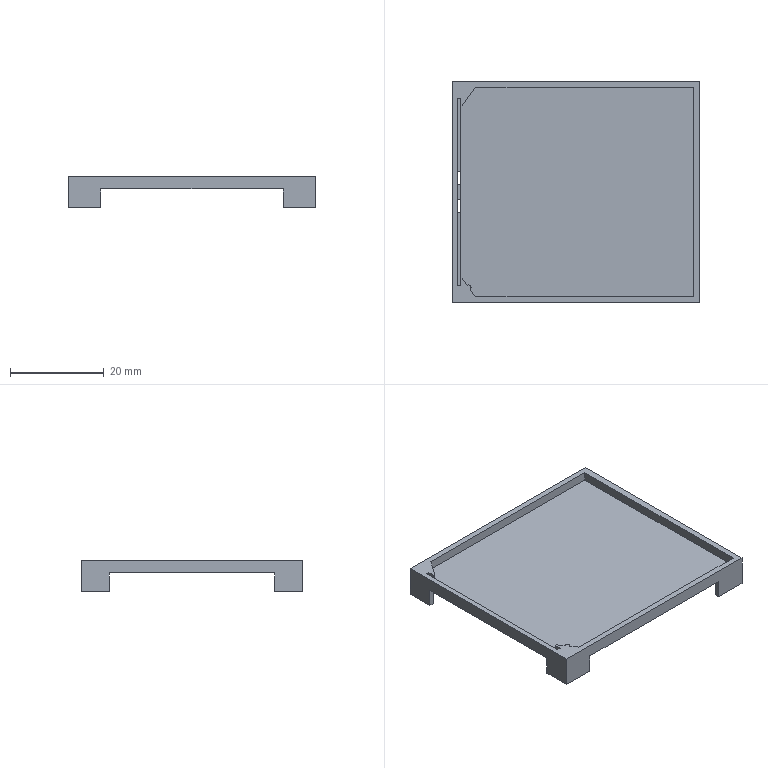Part | NX | features DATUM_CSYS 6, EXTRUDE 5, SKETCH 5 | 1 solid | 49 faces | box 53 x 47.4 x 6.67 mm | volume 2471 mm3 | plane 46 | cylinder 3 | commonest cylinder face diameters 0.4 x2 1 x1
STEP:
#1=CARTESIAN_POINT('',(1.15,25.4,0.35));
#2=VERTEX_POINT('',#1);
#3=CARTESIAN_POINT('',(1.85,25.4,0.35));
#4=VERTEX_POINT('',#3);
#5=CARTESIAN_POINT('',(1.15,25.4,0.35));
#6=DIRECTION('',(1.,0.,0.));
#7=VECTOR('',#6,1000.);
#8=LINE('',#5,#7);
#9=EDGE_CURVE('',#2,#4,#8,.T.);
#10=ORIENTED_EDGE('',*,*,#9,.F.);
#11=CARTESIAN_POINT('',(1.15,22.,0.35));
#12=VERTEX_POINT('',#11);
#13=CARTESIAN_POINT('',(1.15,43.6,0.35));
#14=DIRECTION('',(0.,-1.,0.));
#15=VECTOR('',#14,1000.);
#16=LINE('',#13,#15);
#17=EDGE_CURVE('',#2,#12,#16,.T.);
#18=ORIENTED_EDGE('',*,*,#17,.T.);
#19=CARTESIAN_POINT('',(1.85,22.,0.35));
#20=VERTEX_POINT('',#19);
#21=CARTESIAN_POINT('',(1.85,22.,0.35));
#22=DIRECTION('',(-1.,0.,0.));
#23=VECTOR('',#22,1000.);
#24=LINE('',#21,#23);
#25=EDGE_CURVE('',#20,#12,#24,.T.);
#26=ORIENTED_EDGE('',*,*,#25,.F.);
#27=CARTESIAN_POINT('',(1.85,3.8,0.35));
#28=DIRECTION('',(0.,1.,0.));
#29=VECTOR('',#28,1000.);
#30=LINE('',#27,#29);
#31=EDGE_CURVE('',#20,#4,#30,.T.);
#32=ORIENTED_EDGE('',*,*,#31,.T.);
#33=EDGE_LOOP('',(#10,#18,#26,#32));
#34=FACE_BOUND('',#33,.T.);
#35=CARTESIAN_POINT('',(0.,0.,0.35));
#36=DIRECTION('',(0.,0.,1.));
#37=DIRECTION('',(1.,0.,0.));
#38=AXIS2_PLACEMENT_3D('',#35,#36,#37);
#39=PLANE('',#38);
#40=ADVANCED_FACE('',(#34),#39,.T.);
#41=CARTESIAN_POINT('',(1.15,19.4,0.35));
#42=VERTEX_POINT('',#41);
#43=CARTESIAN_POINT('',(1.85,19.4,0.35));
#44=VERTEX_POINT('',#43);
#45=CARTESIAN_POINT('',(1.15,19.4,0.35));
#46=DIRECTION('',(1.,0.,0.));
#47=VECTOR('',#46,1000.);
#48=LINE('',#45,#47);
#49=EDGE_CURVE('',#42,#44,#48,.T.);
#50=ORIENTED_EDGE('',*,*,#49,.F.);
#51=CARTESIAN_POINT('',(1.15,3.8,0.35));
#52=VERTEX_POINT('',#51);
#53=CARTESIAN_POINT('',(1.15,43.6,0.35));
#54=DIRECTION('',(0.,-1.,0.));
#55=VECTOR('',#54,1000.);
#56=LINE('',#53,#55);
#57=EDGE_CURVE('',#42,#52,#56,.T.);
#58=ORIENTED_EDGE('',*,*,#57,.T.);
#59=CARTESIAN_POINT('',(1.85,3.8,0.35));
#60=VERTEX_POINT('',#59);
#61=CARTESIAN_POINT('',(1.15,3.8,0.35));
#62=DIRECTION('',(1.,0.,0.));
#63=VECTOR('',#62,1000.);
#64=LINE('',#61,#63);
#65=EDGE_CURVE('',#52,#60,#64,.T.);
#66=ORIENTED_EDGE('',*,*,#65,.T.);
#67=CARTESIAN_POINT('',(1.85,3.8,0.35));
#68=DIRECTION('',(0.,1.,0.));
#69=VECTOR('',#68,1000.);
#70=LINE('',#67,#69);
#71=EDGE_CURVE('',#60,#44,#70,.T.);
#72=ORIENTED_EDGE('',*,*,#71,.T.);
#73=EDGE_LOOP('',(#50,#58,#66,#72));
#74=FACE_BOUND('',#73,.T.);
#75=CARTESIAN_POINT('',(0.,0.,0.35));
#76=DIRECTION('',(0.,0.,1.));
#77=DIRECTION('',(1.,0.,0.));
#78=AXIS2_PLACEMENT_3D('',#75,#76,#77);
#79=PLANE('',#78);
#80=ADVANCED_FACE('',(#74),#79,.T.);
#81=CARTESIAN_POINT('',(1.85,28.,0.));
#82=VERTEX_POINT('',#81);
#83=CARTESIAN_POINT('',(1.15,28.,0.));
#84=VERTEX_POINT('',#83);
#85=CARTESIAN_POINT('',(0.,28.,0.));
#86=DIRECTION('',(-1.,0.,0.));
#87=VECTOR('',#86,1000.);
#88=LINE('',#85,#87);
#89=EDGE_CURVE('',#82,#84,#88,.T.);
#90=ORIENTED_EDGE('',*,*,#89,.T.);
#91=CARTESIAN_POINT('',(1.15,25.4,0.));
#92=VERTEX_POINT('',#91);
#93=CARTESIAN_POINT('',(1.15,0.,0.));
#94=DIRECTION('',(0.,-1.,0.));
#95=VECTOR('',#94,1000.);
#96=LINE('',#93,#95);
#97=EDGE_CURVE('',#84,#92,#96,.T.);
#98=ORIENTED_EDGE('',*,*,#97,.T.);
#99=CARTESIAN_POINT('',(1.85,25.4,0.));
#100=VERTEX_POINT('',#99);
#101=CARTESIAN_POINT('',(0.,25.4,0.));
#102=DIRECTION('',(1.,0.,0.));
#103=VECTOR('',#102,1000.);
#104=LINE('',#101,#103);
#105=EDGE_CURVE('',#92,#100,#104,.T.);
#106=ORIENTED_EDGE('',*,*,#105,.T.);
#107=CARTESIAN_POINT('',(1.85,0.,0.));
#108=DIRECTION('',(0.,1.,0.));
#109=VECTOR('',#108,1000.);
#110=LINE('',#107,#109);
#111=EDGE_CURVE('',#100,#82,#110,.T.);
#112=ORIENTED_EDGE('',*,*,#111,.T.);
#113=EDGE_LOOP('',(#90,#98,#106,#112));
#114=FACE_BOUND('',#113,.T.);
#115=CARTESIAN_POINT('',(1.85,22.,0.));
#116=VERTEX_POINT('',#115);
#117=CARTESIAN_POINT('',(1.15,22.,0.));
#118=VERTEX_POINT('',#117);
#119=CARTESIAN_POINT('',(0.,22.,0.));
#120=DIRECTION('',(-1.,0.,0.));
#121=VECTOR('',#120,1000.);
#122=LINE('',#119,#121);
#123=EDGE_CURVE('',#116,#118,#122,.T.);
#124=ORIENTED_EDGE('',*,*,#123,.T.);
#125=CARTESIAN_POINT('',(1.15,19.4,0.));
#126=VERTEX_POINT('',#125);
#127=CARTESIAN_POINT('',(1.15,0.,0.));
#128=DIRECTION('',(0.,-1.,0.));
#129=VECTOR('',#128,1000.);
#130=LINE('',#127,#129);
#131=EDGE_CURVE('',#118,#126,#130,.T.);
#132=ORIENTED_EDGE('',*,*,#131,.T.);
#133=CARTESIAN_POINT('',(1.85,19.4,0.));
#134=VERTEX_POINT('',#133);
#135=CARTESIAN_POINT('',(0.,19.4,0.));
#136=DIRECTION('',(1.,0.,0.));
#137=VECTOR('',#136,1000.);
#138=LINE('',#135,#137);
#139=EDGE_CURVE('',#126,#134,#138,.T.);
#140=ORIENTED_EDGE('',*,*,#139,.T.);
#141=CARTESIAN_POINT('',(1.85,0.,0.));
#142=DIRECTION('',(0.,1.,0.));
#143=VECTOR('',#142,1000.);
#144=LINE('',#141,#143);
#145=EDGE_CURVE('',#134,#116,#144,.T.);
#146=ORIENTED_EDGE('',*,*,#145,.T.);
#147=EDGE_LOOP('',(#124,#132,#140,#146));
#148=FACE_BOUND('',#147,.T.);
#149=CARTESIAN_POINT('',(46.,46.4,0.));
#150=VERTEX_POINT('',#149);
#151=CARTESIAN_POINT('',(46.,47.4,0.));
#152=VERTEX_POINT('',#151);
#153=CARTESIAN_POINT('',(46.,46.4,0.));
#154=DIRECTION('',(0.,1.,0.));
#155=VECTOR('',#154,1000.);
#156=LINE('',#153,#155);
#157=EDGE_CURVE('',#150,#152,#156,.T.);
#158=ORIENTED_EDGE('',*,*,#157,.F.);
#159=CARTESIAN_POINT('',(52.,46.4,0.));
#160=VERTEX_POINT('',#159);
#161=CARTESIAN_POINT('',(52.,46.4,0.));
#162=DIRECTION('',(-1.,0.,0.));
#163=VECTOR('',#162,1000.);
#164=LINE('',#161,#163);
#165=EDGE_CURVE('',#160,#150,#164,.T.);
#166=ORIENTED_EDGE('',*,*,#165,.F.);
#167=CARTESIAN_POINT('',(52.,41.4,0.));
#168=VERTEX_POINT('',#167);
#169=CARTESIAN_POINT('',(52.,41.4,0.));
#170=DIRECTION('',(0.,1.,0.));
#171=VECTOR('',#170,1000.);
#172=LINE('',#169,#171);
#173=EDGE_CURVE('',#168,#160,#172,.T.);
#174=ORIENTED_EDGE('',*,*,#173,.F.);
#175=CARTESIAN_POINT('',(53.,41.4,0.));
#176=VERTEX_POINT('',#175);
#177=CARTESIAN_POINT('',(53.,41.4,0.));
#178=DIRECTION('',(-1.,0.,0.));
#179=VECTOR('',#178,1000.);
#180=LINE('',#177,#179);
#181=EDGE_CURVE('',#176,#168,#180,.T.);
#182=ORIENTED_EDGE('',*,*,#181,.F.);
#183=CARTESIAN_POINT('',(53.,6.,0.));
#184=VERTEX_POINT('',#183);
#185=CARTESIAN_POINT('',(53.,0.,0.));
#186=DIRECTION('',(0.,1.,0.));
#187=VECTOR('',#186,1000.);
#188=LINE('',#185,#187);
#189=EDGE_CURVE('',#184,#176,#188,.T.);
#190=ORIENTED_EDGE('',*,*,#189,.F.);
#191=CARTESIAN_POINT('',(52.,6.,0.));
#192=VERTEX_POINT('',#191);
#193=CARTESIAN_POINT('',(52.,6.,0.));
#194=DIRECTION('',(1.,0.,0.));
#195=VECTOR('',#194,1000.);
#196=LINE('',#193,#195);
#197=EDGE_CURVE('',#192,#184,#196,.T.);
#198=ORIENTED_EDGE('',*,*,#197,.F.);
#199=CARTESIAN_POINT('',(52.,1.,0.));
#200=VERTEX_POINT('',#199);
#201=CARTESIAN_POINT('',(52.,1.,0.));
#202=DIRECTION('',(0.,1.,0.));
#203=VECTOR('',#202,1000.);
#204=LINE('',#201,#203);
#205=EDGE_CURVE('',#200,#192,#204,.T.);
#206=ORIENTED_EDGE('',*,*,#205,.F.);
#207=CARTESIAN_POINT('',(46.,1.,0.));
#208=VERTEX_POINT('',#207);
#209=CARTESIAN_POINT('',(46.,1.,0.));
#210=DIRECTION('',(1.,0.,0.));
#211=VECTOR('',#210,1000.);
#212=LINE('',#209,#211);
#213=EDGE_CURVE('',#208,#200,#212,.T.);
#214=ORIENTED_EDGE('',*,*,#213,.F.);
#215=CARTESIAN_POINT('',(46.,0.,0.));
#216=VERTEX_POINT('',#215);
#217=CARTESIAN_POINT('',(46.,0.,0.));
#218=DIRECTION('',(0.,1.,0.));
#219=VECTOR('',#218,1000.);
#220=LINE('',#217,#219);
#221=EDGE_CURVE('',#216,#208,#220,.T.);
#222=ORIENTED_EDGE('',*,*,#221,.F.);
#223=CARTESIAN_POINT('',(7.,0.,0.));
#224=VERTEX_POINT('',#223);
#225=CARTESIAN_POINT('',(0.,0.,0.));
#226=DIRECTION('',(1.,0.,0.));
#227=VECTOR('',#226,1000.);
#228=LINE('',#225,#227);
#229=EDGE_CURVE('',#224,#216,#228,.T.);
#230=ORIENTED_EDGE('',*,*,#229,.F.);
#231=CARTESIAN_POINT('',(7.,1.,0.));
#232=VERTEX_POINT('',#231);
#233=CARTESIAN_POINT('',(7.,1.,0.));
#234=DIRECTION('',(0.,-1.,0.));
#235=VECTOR('',#234,1000.);
#236=LINE('',#233,#235);
#237=EDGE_CURVE('',#232,#224,#236,.T.);
#238=ORIENTED_EDGE('',*,*,#237,.F.);
#239=CARTESIAN_POINT('',(1.,1.,0.));
#240=VERTEX_POINT('',#239);
#241=CARTESIAN_POINT('',(1.,1.,0.));
#242=DIRECTION('',(1.,0.,0.));
#243=VECTOR('',#242,1000.);
#244=LINE('',#241,#243);
#245=EDGE_CURVE('',#240,#232,#244,.T.);
#246=ORIENTED_EDGE('',*,*,#245,.F.);
#247=CARTESIAN_POINT('',(1.,6.,0.));
#248=VERTEX_POINT('',#247);
#249=CARTESIAN_POINT('',(1.,6.,0.));
#250=DIRECTION('',(0.,-1.,0.));
#251=VECTOR('',#250,1000.);
#252=LINE('',#249,#251);
#253=EDGE_CURVE('',#248,#240,#252,.T.);
#254=ORIENTED_EDGE('',*,*,#253,.F.);
#255=CARTESIAN_POINT('',(0.,6.,0.));
#256=VERTEX_POINT('',#255);
#257=CARTESIAN_POINT('',(0.,6.,0.));
#258=DIRECTION('',(1.,0.,0.));
#259=VECTOR('',#258,1000.);
#260=LINE('',#257,#259);
#261=EDGE_CURVE('',#256,#248,#260,.T.);
#262=ORIENTED_EDGE('',*,*,#261,.F.);
#263=CARTESIAN_POINT('',(0.,41.4,0.));
#264=VERTEX_POINT('',#263);
#265=CARTESIAN_POINT('',(0.,47.4,0.));
#266=DIRECTION('',(0.,-1.,0.));
#267=VECTOR('',#266,1000.);
#268=LINE('',#265,#267);
#269=EDGE_CURVE('',#264,#256,#268,.T.);
#270=ORIENTED_EDGE('',*,*,#269,.F.);
#271=CARTESIAN_POINT('',(1.,41.4,0.));
#272=VERTEX_POINT('',#271);
#273=CARTESIAN_POINT('',(1.,41.4,0.));
#274=DIRECTION('',(-1.,0.,0.));
#275=VECTOR('',#274,1000.);
#276=LINE('',#273,#275);
#277=EDGE_CURVE('',#272,#264,#276,.T.);
#278=ORIENTED_EDGE('',*,*,#277,.F.);
#279=CARTESIAN_POINT('',(1.,46.4,0.));
#280=VERTEX_POINT('',#279);
#281=CARTESIAN_POINT('',(1.,46.4,0.));
#282=DIRECTION('',(0.,-1.,0.));
#283=VECTOR('',#282,1000.);
#284=LINE('',#281,#283);
#285=EDGE_CURVE('',#280,#272,#284,.T.);
#286=ORIENTED_EDGE('',*,*,#285,.F.);
#287=CARTESIAN_POINT('',(7.,46.4,0.));
#288=VERTEX_POINT('',#287);
#289=CARTESIAN_POINT('',(7.,46.4,0.));
#290=DIRECTION('',(-1.,0.,0.));
#291=VECTOR('',#290,1000.);
#292=LINE('',#289,#291);
#293=EDGE_CURVE('',#288,#280,#292,.T.);
#294=ORIENTED_EDGE('',*,*,#293,.F.);
#295=CARTESIAN_POINT('',(7.,47.4,0.));
#296=VERTEX_POINT('',#295);
#297=CARTESIAN_POINT('',(7.,47.4,0.));
#298=DIRECTION('',(0.,-1.,0.));
#299=VECTOR('',#298,1000.);
#300=LINE('',#297,#299);
#301=EDGE_CURVE('',#296,#288,#300,.T.);
#302=ORIENTED_EDGE('',*,*,#301,.F.);
#303=CARTESIAN_POINT('',(53.,47.4,0.));
#304=DIRECTION('',(-1.,0.,0.));
#305=VECTOR('',#304,1000.);
#306=LINE('',#303,#305);
#307=EDGE_CURVE('',#152,#296,#306,.T.);
#308=ORIENTED_EDGE('',*,*,#307,.F.);
#309=EDGE_LOOP('',(#158,#166,#174,#182,#190,#198,#206,#214,#222,#230,#238,#246,#254,#262,#270,#278,#286,#294,#302,#308));
#310=FACE_BOUND('',#309,.T.);
#311=CARTESIAN_POINT('',(0.,0.,0.));
#312=DIRECTION('',(0.,0.,1.));
#313=DIRECTION('',(1.,0.,0.));
#314=AXIS2_PLACEMENT_3D('',#311,#312,#313);
#315=PLANE('',#314);
#316=ADVANCED_FACE('',(#114,#148,#310),#315,.F.);
#317=CARTESIAN_POINT('',(0.,47.4,2.67));
#318=VERTEX_POINT('',#317);
#319=CARTESIAN_POINT('',(0.,47.4,-4.));
#320=VERTEX_POINT('',#319);
#321=CARTESIAN_POINT('',(0.,47.4,2.67));
#322=DIRECTION('',(0.,0.,-1.));
#323=VECTOR('',#322,1000.);
#324=LINE('',#321,#323);
#325=EDGE_CURVE('',#318,#320,#324,.T.);
#326=ORIENTED_EDGE('',*,*,#325,.T.);
#327=CARTESIAN_POINT('',(0.,41.4,-4.));
#328=VERTEX_POINT('',#327);
#329=CARTESIAN_POINT('',(0.,41.4,-4.));
#330=DIRECTION('',(0.,1.,0.));
#331=VECTOR('',#330,1000.);
#332=LINE('',#329,#331);
#333=EDGE_CURVE('',#328,#320,#332,.T.);
#334=ORIENTED_EDGE('',*,*,#333,.F.);
#335=CARTESIAN_POINT('',(0.,41.4,-4.));
#336=DIRECTION('',(0.,0.,1.));
#337=VECTOR('',#336,1000.);
#338=LINE('',#335,#337);
#339=EDGE_CURVE('',#328,#264,#338,.T.);
#340=ORIENTED_EDGE('',*,*,#339,.T.);
#341=ORIENTED_EDGE('',*,*,#269,.T.);
#342=CARTESIAN_POINT('',(0.,6.,-4.));
#343=VERTEX_POINT('',#342);
#344=CARTESIAN_POINT('',(0.,6.,-4.));
#345=DIRECTION('',(0.,0.,1.));
#346=VECTOR('',#345,1000.);
#347=LINE('',#344,#346);
#348=EDGE_CURVE('',#343,#256,#347,.T.);
#349=ORIENTED_EDGE('',*,*,#348,.F.);
#350=CARTESIAN_POINT('',(0.,0.,-4.));
#351=VERTEX_POINT('',#350);
#352=CARTESIAN_POINT('',(0.,0.,-4.));
#353=DIRECTION('',(0.,1.,0.));
#354=VECTOR('',#353,1000.);
#355=LINE('',#352,#354);
#356=EDGE_CURVE('',#351,#343,#355,.T.);
#357=ORIENTED_EDGE('',*,*,#356,.F.);
#358=CARTESIAN_POINT('',(0.,0.,2.67));
#359=VERTEX_POINT('',#358);
#360=CARTESIAN_POINT('',(0.,0.,2.67));
#361=DIRECTION('',(0.,0.,-1.));
#362=VECTOR('',#361,1000.);
#363=LINE('',#360,#362);
#364=EDGE_CURVE('',#359,#351,#363,.T.);
#365=ORIENTED_EDGE('',*,*,#364,.F.);
#366=CARTESIAN_POINT('',(0.,47.4,2.67));
#367=DIRECTION('',(0.,-1.,0.));
#368=VECTOR('',#367,1000.);
#369=LINE('',#366,#368);
#370=EDGE_CURVE('',#318,#359,#369,.T.);
#371=ORIENTED_EDGE('',*,*,#370,.F.);
#372=EDGE_LOOP('',(#326,#334,#340,#341,#349,#357,#365,#371));
#373=FACE_BOUND('',#372,.T.);
#374=CARTESIAN_POINT('',(0.,47.4,2.67));
#375=DIRECTION('',(1.,0.,0.));
#376=DIRECTION('',(0.,1.,0.));
#377=AXIS2_PLACEMENT_3D('',#374,#375,#376);
#378=PLANE('',#377);
#379=ADVANCED_FACE('',(#373),#378,.F.);
#380=ORIENTED_EDGE('',*,*,#364,.T.);
#381=CARTESIAN_POINT('',(7.,0.,-4.));
#382=VERTEX_POINT('',#381);
#383=CARTESIAN_POINT('',(7.,0.,-4.));
#384=DIRECTION('',(-1.,0.,0.));
#385=VECTOR('',#384,1000.);
#386=LINE('',#383,#385);
#387=EDGE_CURVE('',#382,#351,#386,.T.);
#388=ORIENTED_EDGE('',*,*,#387,.F.);
#389=CARTESIAN_POINT('',(7.,0.,-4.));
#390=DIRECTION('',(0.,0.,1.));
#391=VECTOR('',#390,1000.);
#392=LINE('',#389,#391);
#393=EDGE_CURVE('',#382,#224,#392,.T.);
#394=ORIENTED_EDGE('',*,*,#393,.T.);
#395=ORIENTED_EDGE('',*,*,#229,.T.);
#396=CARTESIAN_POINT('',(46.,0.,-4.));
#397=VERTEX_POINT('',#396);
#398=CARTESIAN_POINT('',(46.,0.,-4.));
#399=DIRECTION('',(0.,0.,1.));
#400=VECTOR('',#399,1000.);
#401=LINE('',#398,#400);
#402=EDGE_CURVE('',#397,#216,#401,.T.);
#403=ORIENTED_EDGE('',*,*,#402,.F.);
#404=CARTESIAN_POINT('',(53.,0.,-4.));
#405=VERTEX_POINT('',#404);
#406=CARTESIAN_POINT('',(53.,0.,-4.));
#407=DIRECTION('',(-1.,0.,0.));
#408=VECTOR('',#407,1000.);
#409=LINE('',#406,#408);
#410=EDGE_CURVE('',#405,#397,#409,.T.);
#411=ORIENTED_EDGE('',*,*,#410,.F.);
#412=CARTESIAN_POINT('',(53.,0.,2.67));
#413=VERTEX_POINT('',#412);
#414=CARTESIAN_POINT('',(53.,0.,2.67));
#415=DIRECTION('',(0.,0.,-1.));
#416=VECTOR('',#415,1000.);
#417=LINE('',#414,#416);
#418=EDGE_CURVE('',#413,#405,#417,.T.);
#419=ORIENTED_EDGE('',*,*,#418,.F.);
#420=CARTESIAN_POINT('',(0.,0.,2.67));
#421=DIRECTION('',(1.,0.,0.));
#422=VECTOR('',#421,1000.);
#423=LINE('',#420,#422);
#424=EDGE_CURVE('',#359,#413,#423,.T.);
#425=ORIENTED_EDGE('',*,*,#424,.F.);
#426=EDGE_LOOP('',(#380,#388,#394,#395,#403,#411,#419,#425));
#427=FACE_BOUND('',#426,.T.);
#428=CARTESIAN_POINT('',(0.,0.,2.67));
#429=DIRECTION('',(0.,1.,0.));
#430=DIRECTION('',(0.,0.,1.));
#431=AXIS2_PLACEMENT_3D('',#428,#429,#430);
#432=PLANE('',#431);
#433=ADVANCED_FACE('',(#427),#432,.F.);
#434=ORIENTED_EDGE('',*,*,#418,.T.);
#435=CARTESIAN_POINT('',(53.,6.,-4.));
#436=VERTEX_POINT('',#435);
#437=CARTESIAN_POINT('',(53.,6.,-4.));
#438=DIRECTION('',(0.,-1.,0.));
#439=VECTOR('',#438,1000.);
#440=LINE('',#437,#439);
#441=EDGE_CURVE('',#436,#405,#440,.T.);
#442=ORIENTED_EDGE('',*,*,#441,.F.);
#443=CARTESIAN_POINT('',(53.,6.,-4.));
#444=DIRECTION('',(0.,0.,1.));
#445=VECTOR('',#444,1000.);
#446=LINE('',#443,#445);
#447=EDGE_CURVE('',#436,#184,#446,.T.);
#448=ORIENTED_EDGE('',*,*,#447,.T.);
#449=ORIENTED_EDGE('',*,*,#189,.T.);
#450=CARTESIAN_POINT('',(53.,41.4,-4.));
#451=VERTEX_POINT('',#450);
#452=CARTESIAN_POINT('',(53.,41.4,-4.));
#453=DIRECTION('',(0.,0.,1.));
#454=VECTOR('',#453,1000.);
#455=LINE('',#452,#454);
#456=EDGE_CURVE('',#451,#176,#455,.T.);
#457=ORIENTED_EDGE('',*,*,#456,.F.);
#458=CARTESIAN_POINT('',(53.,47.4,-4.));
#459=VERTEX_POINT('',#458);
#460=CARTESIAN_POINT('',(53.,47.4,-4.));
#461=DIRECTION('',(0.,-1.,0.));
#462=VECTOR('',#461,1000.);
#463=LINE('',#460,#462);
#464=EDGE_CURVE('',#459,#451,#463,.T.);
#465=ORIENTED_EDGE('',*,*,#464,.F.);
#466=CARTESIAN_POINT('',(53.,47.4,2.67));
#467=VERTEX_POINT('',#466);
#468=CARTESIAN_POINT('',(53.,47.4,2.67));
#469=DIRECTION('',(0.,0.,-1.));
#470=VECTOR('',#469,1000.);
#471=LINE('',#468,#470);
#472=EDGE_CURVE('',#467,#459,#471,.T.);
#473=ORIENTED_EDGE('',*,*,#472,.F.);
#474=CARTESIAN_POINT('',(53.,0.,2.67));
#475=DIRECTION('',(0.,1.,0.));
#476=VECTOR('',#475,1000.);
#477=LINE('',#474,#476);
#478=EDGE_CURVE('',#413,#467,#477,.T.);
#479=ORIENTED_EDGE('',*,*,#478,.F.);
#480=EDGE_LOOP('',(#434,#442,#448,#449,#457,#465,#473,#479));
#481=FACE_BOUND('',#480,.T.);
#482=CARTESIAN_POINT('',(53.,0.,2.67));
#483=DIRECTION('',(-1.,0.,0.));
#484=DIRECTION('',(0.,0.,1.));
#485=AXIS2_PLACEMENT_3D('',#482,#483,#484);
#486=PLANE('',#485);
#487=ADVANCED_FACE('',(#481),#486,.F.);
#488=ORIENTED_EDGE('',*,*,#472,.T.);
#489=CARTESIAN_POINT('',(46.,47.4,-4.));
#490=VERTEX_POINT('',#489);
#491=CARTESIAN_POINT('',(46.,47.4,-4.));
#492=DIRECTION('',(1.,0.,0.));
#493=VECTOR('',#492,1000.);
#494=LINE('',#491,#493);
#495=EDGE_CURVE('',#490,#459,#494,.T.);
#496=ORIENTED_EDGE('',*,*,#495,.F.);
#497=CARTESIAN_POINT('',(46.,47.4,-4.));
#498=DIRECTION('',(0.,0.,1.));
#499=VECTOR('',#498,1000.);
#500=LINE('',#497,#499);
#501=EDGE_CURVE('',#490,#152,#500,.T.);
#502=ORIENTED_EDGE('',*,*,#501,.T.);
#503=ORIENTED_EDGE('',*,*,#307,.T.);
#504=CARTESIAN_POINT('',(7.,47.4,-4.));
#505=VERTEX_POINT('',#504);
#506=CARTESIAN_POINT('',(7.,47.4,-4.));
#507=DIRECTION('',(0.,0.,1.));
#508=VECTOR('',#507,1000.);
#509=LINE('',#506,#508);
#510=EDGE_CURVE('',#505,#296,#509,.T.);
#511=ORIENTED_EDGE('',*,*,#510,.F.);
#512=CARTESIAN_POINT('',(0.,47.4,-4.));
#513=DIRECTION('',(1.,0.,0.));
#514=VECTOR('',#513,1000.);
#515=LINE('',#512,#514);
#516=EDGE_CURVE('',#320,#505,#515,.T.);
#517=ORIENTED_EDGE('',*,*,#516,.F.);
#518=ORIENTED_EDGE('',*,*,#325,.F.);
#519=CARTESIAN_POINT('',(53.,47.4,2.67));
#520=DIRECTION('',(-1.,0.,0.));
#521=VECTOR('',#520,1000.);
#522=LINE('',#519,#521);
#523=EDGE_CURVE('',#467,#318,#522,.T.);
#524=ORIENTED_EDGE('',*,*,#523,.F.);
#525=EDGE_LOOP('',(#488,#496,#502,#503,#511,#517,#518,#524));
#526=FACE_BOUND('',#525,.T.);
#527=CARTESIAN_POINT('',(53.,47.4,2.67));
#528=DIRECTION('',(0.,-1.,0.));
#529=DIRECTION('',(1.,0.,0.));
#530=AXIS2_PLACEMENT_3D('',#527,#528,#529);
#531=PLANE('',#530);
#532=ADVANCED_FACE('',(#526),#531,.F.);
#533=CARTESIAN_POINT('',(1.15,43.6,2.67));
#534=VERTEX_POINT('',#533);
#535=CARTESIAN_POINT('',(1.15,3.8,2.67));
#536=VERTEX_POINT('',#535);
#537=CARTESIAN_POINT('',(1.15,43.6,2.67));
#538=DIRECTION('',(0.,-1.,0.));
#539=VECTOR('',#538,1000.);
#540=LINE('',#537,#539);
#541=EDGE_CURVE('',#534,#536,#540,.T.);
#542=ORIENTED_EDGE('',*,*,#541,.F.);
#543=CARTESIAN_POINT('',(1.85,43.6,2.67));
#544=VERTEX_POINT('',#543);
#545=CARTESIAN_POINT('',(1.85,43.6,2.67));
#546=DIRECTION('',(-1.,0.,0.));
#547=VECTOR('',#546,1000.);
#548=LINE('',#545,#547);
#549=EDGE_CURVE('',#544,#534,#548,.T.);
#550=ORIENTED_EDGE('',*,*,#549,.F.);
#551=CARTESIAN_POINT('',(1.85,42.1,2.67));
#552=VERTEX_POINT('',#551);
#553=CARTESIAN_POINT('',(1.85,42.1,2.67));
#554=DIRECTION('',(0.,1.,0.));
#555=VECTOR('',#554,1000.);
#556=LINE('',#553,#555);
#557=EDGE_CURVE('',#552,#544,#556,.T.);
#558=ORIENTED_EDGE('',*,*,#557,.F.);
#559=CARTESIAN_POINT('',(2.15,42.1,2.67));
#560=VERTEX_POINT('',#559);
#561=CARTESIAN_POINT('',(2.15,42.1,2.67));
#562=DIRECTION('',(-1.,0.,0.));
#563=VECTOR('',#562,1000.);
#564=LINE('',#561,#563);
#565=EDGE_CURVE('',#560,#552,#564,.T.);
#566=ORIENTED_EDGE('',*,*,#565,.F.);
#567=CARTESIAN_POINT('',(4.94,46.016,2.67));
#568=VERTEX_POINT('',#567);
#569=CARTESIAN_POINT('',(4.94,46.016,2.67));
#570=DIRECTION('',(-0.5803,-0.8144,0.));
#571=VECTOR('',#570,1000.);
#572=LINE('',#569,#571);
#573=EDGE_CURVE('',#568,#560,#572,.T.);
#574=ORIENTED_EDGE('',*,*,#573,.F.);
#575=CARTESIAN_POINT('',(5.103,46.1,2.67));
#576=VERTEX_POINT('',#575);
#577=CARTESIAN_POINT('',(5.103,45.9,2.67));
#578=DIRECTION('',(0.,0.,1.));
#579=DIRECTION('',(1.,0.,0.));
#580=AXIS2_PLACEMENT_3D('',#577,#578,#579);
#581=CIRCLE('',#580,0.2);
#582=EDGE_CURVE('',#576,#568,#581,.T.);
#583=ORIENTED_EDGE('',*,*,#582,.F.);
#584=CARTESIAN_POINT('',(51.6,46.1,2.67));
#585=VERTEX_POINT('',#584);
#586=CARTESIAN_POINT('',(51.6,46.1,2.67));
#587=DIRECTION('',(-1.,0.,0.));
#588=VECTOR('',#587,1000.);
#589=LINE('',#586,#588);
#590=EDGE_CURVE('',#585,#576,#589,.T.);
#591=ORIENTED_EDGE('',*,*,#590,.F.);
#592=CARTESIAN_POINT('',(51.6,1.3,2.67));
#593=VERTEX_POINT('',#592);
#594=CARTESIAN_POINT('',(51.6,1.3,2.67));
#595=DIRECTION('',(0.,1.,0.));
#596=VECTOR('',#595,1000.);
#597=LINE('',#594,#596);
#598=EDGE_CURVE('',#593,#585,#597,.T.);
#599=ORIENTED_EDGE('',*,*,#598,.F.);
#600=CARTESIAN_POINT('',(5.103,1.3,2.67));
#601=VERTEX_POINT('',#600);
#602=CARTESIAN_POINT('',(5.103,1.3,2.67));
#603=DIRECTION('',(1.,0.,0.));
#604=VECTOR('',#603,1000.);
#605=LINE('',#602,#604);
#606=EDGE_CURVE('',#601,#593,#605,.T.);
#607=ORIENTED_EDGE('',*,*,#606,.F.);
#608=CARTESIAN_POINT('',(4.94,1.384,2.67));
#609=VERTEX_POINT('',#608);
#610=CARTESIAN_POINT('',(5.103,1.5,2.67));
#611=DIRECTION('',(0.,0.,1.));
#612=DIRECTION('',(1.,0.,0.));
#613=AXIS2_PLACEMENT_3D('',#610,#611,#612);
#614=CIRCLE('',#613,0.2);
#615=EDGE_CURVE('',#609,#601,#614,.T.);
#616=ORIENTED_EDGE('',*,*,#615,.F.);
#617=CARTESIAN_POINT('',(3.84,2.928,2.67));
#618=VERTEX_POINT('',#617);
#619=CARTESIAN_POINT('',(3.84,2.928,2.67));
#620=DIRECTION('',(0.5803,-0.8144,0.));
#621=VECTOR('',#620,1000.);
#622=LINE('',#619,#621);
#623=EDGE_CURVE('',#618,#609,#622,.T.);
#624=ORIENTED_EDGE('',*,*,#623,.F.);
#625=CARTESIAN_POINT('',(3.26,3.742,2.67));
#626=VERTEX_POINT('',#625);
#627=CARTESIAN_POINT('',(3.55,3.335,2.67));
#628=DIRECTION('',(0.,0.,-1.));
#629=DIRECTION('',(1.,0.,0.));
#630=AXIS2_PLACEMENT_3D('',#627,#628,#629);
#631=CIRCLE('',#630,0.5);
#632=EDGE_CURVE('',#626,#618,#631,.T.);
#633=ORIENTED_EDGE('',*,*,#632,.F.);
#634=CARTESIAN_POINT('',(2.15,5.3,2.67));
#635=VERTEX_POINT('',#634);
#636=CARTESIAN_POINT('',(2.15,5.3,2.67));
#637=DIRECTION('',(0.5803,-0.8144,0.));
#638=VECTOR('',#637,1000.);
#639=LINE('',#636,#638);
#640=EDGE_CURVE('',#635,#626,#639,.T.);
#641=ORIENTED_EDGE('',*,*,#640,.F.);
#642=CARTESIAN_POINT('',(1.85,5.3,2.67));
#643=VERTEX_POINT('',#642);
#644=CARTESIAN_POINT('',(1.85,5.3,2.67));
#645=DIRECTION('',(1.,0.,0.));
#646=VECTOR('',#645,1000.);
#647=LINE('',#644,#646);
#648=EDGE_CURVE('',#643,#635,#647,.T.);
#649=ORIENTED_EDGE('',*,*,#648,.F.);
#650=CARTESIAN_POINT('',(1.85,3.8,2.67));
#651=VERTEX_POINT('',#650);
#652=CARTESIAN_POINT('',(1.85,3.8,2.67));
#653=DIRECTION('',(0.,1.,0.));
#654=VECTOR('',#653,1000.);
#655=LINE('',#652,#654);
#656=EDGE_CURVE('',#651,#643,#655,.T.);
#657=ORIENTED_EDGE('',*,*,#656,.F.);
#658=CARTESIAN_POINT('',(1.15,3.8,2.67));
#659=DIRECTION('',(1.,0.,0.));
#660=VECTOR('',#659,1000.);
#661=LINE('',#658,#660);
#662=EDGE_CURVE('',#536,#651,#661,.T.);
#663=ORIENTED_EDGE('',*,*,#662,.F.);
#664=EDGE_LOOP('',(#542,#550,#558,#566,#574,#583,#591,#599,#607,#616,#624,#633,#641,#649,#657,#663));
#665=FACE_BOUND('',#664,.T.);
#666=ORIENTED_EDGE('',*,*,#370,.T.);
#667=ORIENTED_EDGE('',*,*,#424,.T.);
#668=ORIENTED_EDGE('',*,*,#478,.T.);
#669=ORIENTED_EDGE('',*,*,#523,.T.);
#670=EDGE_LOOP('',(#666,#667,#668,#669));
#671=FACE_BOUND('',#670,.T.);
#672=CARTESIAN_POINT('',(0.,0.,2.67));
#673=DIRECTION('',(0.,0.,1.));
#674=DIRECTION('',(1.,0.,0.));
#675=AXIS2_PLACEMENT_3D('',#672,#673,#674);
#676=PLANE('',#675);
#677=ADVANCED_FACE('',(#665,#671),#676,.T.);
#678=ORIENTED_EDGE('',*,*,#261,.T.);
#679=CARTESIAN_POINT('',(1.,6.,-4.));
#680=VERTEX_POINT('',#679);
#681=CARTESIAN_POINT('',(1.,6.,-4.));
#682=DIRECTION('',(0.,0.,1.));
#683=VECTOR('',#682,1000.);
#684=LINE('',#681,#683);
#685=EDGE_CURVE('',#680,#248,#684,.T.);
#686=ORIENTED_EDGE('',*,*,#685,.F.);
#687=CARTESIAN_POINT('',(0.,6.,-4.));
#688=DIRECTION('',(1.,0.,0.));
#689=VECTOR('',#688,1000.);
#690=LINE('',#687,#689);
#691=EDGE_CURVE('',#343,#680,#690,.T.);
#692=ORIENTED_EDGE('',*,*,#691,.F.);
#693=ORIENTED_EDGE('',*,*,#348,.T.);
#694=EDGE_LOOP('',(#678,#686,#692,#693));
#695=FACE_BOUND('',#694,.T.);
#696=CARTESIAN_POINT('',(0.,6.,-4.));
#697=DIRECTION('',(0.,-1.,0.));
#698=DIRECTION('',(0.,0.,-1.));
#699=AXIS2_PLACEMENT_3D('',#696,#697,#698);
#700=PLANE('',#699);
#701=ADVANCED_FACE('',(#695),#700,.F.);
#702=ORIENTED_EDGE('',*,*,#253,.T.);
#703=CARTESIAN_POINT('',(1.,1.,-4.));
#704=VERTEX_POINT('',#703);
#705=CARTESIAN_POINT('',(1.,1.,-4.));
#706=DIRECTION('',(0.,0.,1.));
#707=VECTOR('',#706,1000.);
#708=LINE('',#705,#707);
#709=EDGE_CURVE('',#704,#240,#708,.T.);
#710=ORIENTED_EDGE('',*,*,#709,.F.);
#711=CARTESIAN_POINT('',(1.,6.,-4.));
#712=DIRECTION('',(0.,-1.,0.));
#713=VECTOR('',#712,1000.);
#714=LINE('',#711,#713);
#715=EDGE_CURVE('',#680,#704,#714,.T.);
#716=ORIENTED_EDGE('',*,*,#715,.F.);
#717=ORIENTED_EDGE('',*,*,#685,.T.);
#718=EDGE_LOOP('',(#702,#710,#716,#717));
#719=FACE_BOUND('',#718,.T.);
#720=CARTESIAN_POINT('',(1.,6.,-4.));
#721=DIRECTION('',(-1.,0.,0.));
#722=DIRECTION('',(0.,0.,1.));
#723=AXIS2_PLACEMENT_3D('',#720,#721,#722);
#724=PLANE('',#723);
#725=ADVANCED_FACE('',(#719),#724,.F.);
#726=ORIENTED_EDGE('',*,*,#245,.T.);
#727=CARTESIAN_POINT('',(7.,1.,-4.));
#728=VERTEX_POINT('',#727);
#729=CARTESIAN_POINT('',(7.,1.,-4.));
#730=DIRECTION('',(0.,0.,1.));
#731=VECTOR('',#730,1000.);
#732=LINE('',#729,#731);
#733=EDGE_CURVE('',#728,#232,#732,.T.);
#734=ORIENTED_EDGE('',*,*,#733,.F.);
#735=CARTESIAN_POINT('',(1.,1.,-4.));
#736=DIRECTION('',(1.,0.,0.));
#737=VECTOR('',#736,1000.);
#738=LINE('',#735,#737);
#739=EDGE_CURVE('',#704,#728,#738,.T.);
#740=ORIENTED_EDGE('',*,*,#739,.F.);
#741=ORIENTED_EDGE('',*,*,#709,.T.);
#742=EDGE_LOOP('',(#726,#734,#740,#741));
#743=FACE_BOUND('',#742,.T.);
#744=CARTESIAN_POINT('',(1.,1.,-4.));
#745=DIRECTION('',(0.,-1.,0.));
#746=DIRECTION('',(0.,0.,-1.));
#747=AXIS2_PLACEMENT_3D('',#744,#745,#746);
#748=PLANE('',#747);
#749=ADVANCED_FACE('',(#743),#748,.F.);
#750=ORIENTED_EDGE('',*,*,#237,.T.);
#751=ORIENTED_EDGE('',*,*,#393,.F.);
#752=CARTESIAN_POINT('',(7.,1.,-4.));
#753=DIRECTION('',(0.,-1.,0.));
#754=VECTOR('',#753,1000.);
#755=LINE('',#752,#754);
#756=EDGE_CURVE('',#728,#382,#755,.T.);
#757=ORIENTED_EDGE('',*,*,#756,.F.);
#758=ORIENTED_EDGE('',*,*,#733,.T.);
#759=EDGE_LOOP('',(#750,#751,#757,#758));
#760=FACE_BOUND('',#759,.T.);
#761=CARTESIAN_POINT('',(7.,1.,-4.));
#762=DIRECTION('',(-1.,0.,0.));
#763=DIRECTION('',(0.,0.,1.));
#764=AXIS2_PLACEMENT_3D('',#761,#762,#763);
#765=PLANE('',#764);
#766=ADVANCED_FACE('',(#760),#765,.F.);
#767=ORIENTED_EDGE('',*,*,#356,.T.);
#768=ORIENTED_EDGE('',*,*,#691,.T.);
#769=ORIENTED_EDGE('',*,*,#715,.T.);
#770=ORIENTED_EDGE('',*,*,#739,.T.);
#771=ORIENTED_EDGE('',*,*,#756,.T.);
#772=ORIENTED_EDGE('',*,*,#387,.T.);
#773=EDGE_LOOP('',(#767,#768,#769,#770,#771,#772));
#774=FACE_BOUND('',#773,.T.);
#775=CARTESIAN_POINT('',(0.,0.,-4.));
#776=DIRECTION('',(0.,0.,-1.));
#777=DIRECTION('',(-1.,0.,0.));
#778=AXIS2_PLACEMENT_3D('',#775,#776,#777);
#779=PLANE('',#778);
#780=ADVANCED_FACE('',(#774),#779,.T.);
#781=ORIENTED_EDGE('',*,*,#301,.T.);
#782=CARTESIAN_POINT('',(7.,46.4,-4.));
#783=VERTEX_POINT('',#782);
#784=CARTESIAN_POINT('',(7.,46.4,-4.));
#785=DIRECTION('',(0.,0.,1.));
#786=VECTOR('',#785,1000.);
#787=LINE('',#784,#786);
#788=EDGE_CURVE('',#783,#288,#787,.T.);
#789=ORIENTED_EDGE('',*,*,#788,.F.);
#790=CARTESIAN_POINT('',(7.,47.4,-4.));
#791=DIRECTION('',(0.,-1.,0.));
#792=VECTOR('',#791,1000.);
#793=LINE('',#790,#792);
#794=EDGE_CURVE('',#505,#783,#793,.T.);
#795=ORIENTED_EDGE('',*,*,#794,.F.);
#796=ORIENTED_EDGE('',*,*,#510,.T.);
#797=EDGE_LOOP('',(#781,#789,#795,#796));
#798=FACE_BOUND('',#797,.T.);
#799=CARTESIAN_POINT('',(7.,47.4,-4.));
#800=DIRECTION('',(-1.,0.,0.));
#801=DIRECTION('',(0.,-1.,0.));
#802=AXIS2_PLACEMENT_3D('',#799,#800,#801);
#803=PLANE('',#802);
#804=ADVANCED_FACE('',(#798),#803,.F.);
#805=ORIENTED_EDGE('',*,*,#293,.T.);
#806=CARTESIAN_POINT('',(1.,46.4,-4.));
#807=VERTEX_POINT('',#806);
#808=CARTESIAN_POINT('',(1.,46.4,-4.));
#809=DIRECTION('',(0.,0.,1.));
#810=VECTOR('',#809,1000.);
#811=LINE('',#808,#810);
#812=EDGE_CURVE('',#807,#280,#811,.T.);
#813=ORIENTED_EDGE('',*,*,#812,.F.);
#814=CARTESIAN_POINT('',(7.,46.4,-4.));
#815=DIRECTION('',(-1.,0.,0.));
#816=VECTOR('',#815,1000.);
#817=LINE('',#814,#816);
#818=EDGE_CURVE('',#783,#807,#817,.T.);
#819=ORIENTED_EDGE('',*,*,#818,.F.);
#820=ORIENTED_EDGE('',*,*,#788,.T.);
#821=EDGE_LOOP('',(#805,#813,#819,#820));
#822=FACE_BOUND('',#821,.T.);
#823=CARTESIAN_POINT('',(7.,46.4,-4.));
#824=DIRECTION('',(0.,1.,0.));
#825=DIRECTION('',(-1.,0.,0.));
#826=AXIS2_PLACEMENT_3D('',#823,#824,#825);
#827=PLANE('',#826);
#828=ADVANCED_FACE('',(#822),#827,.F.);
#829=ORIENTED_EDGE('',*,*,#285,.T.);
#830=CARTESIAN_POINT('',(1.,41.4,-4.));
#831=VERTEX_POINT('',#830);
#832=CARTESIAN_POINT('',(1.,41.4,-4.));
#833=DIRECTION('',(0.,0.,1.));
#834=VECTOR('',#833,1000.);
#835=LINE('',#832,#834);
#836=EDGE_CURVE('',#831,#272,#835,.T.);
#837=ORIENTED_EDGE('',*,*,#836,.F.);
#838=CARTESIAN_POINT('',(1.,46.4,-4.));
#839=DIRECTION('',(0.,-1.,0.));
#840=VECTOR('',#839,1000.);
#841=LINE('',#838,#840);
#842=EDGE_CURVE('',#807,#831,#841,.T.);
#843=ORIENTED_EDGE('',*,*,#842,.F.);
#844=ORIENTED_EDGE('',*,*,#812,.T.);
#845=EDGE_LOOP('',(#829,#837,#843,#844));
#846=FACE_BOUND('',#845,.T.);
#847=CARTESIAN_POINT('',(1.,46.4,-4.));
#848=DIRECTION('',(-1.,0.,0.));
#849=DIRECTION('',(0.,-1.,0.));
#850=AXIS2_PLACEMENT_3D('',#847,#848,#849);
#851=PLANE('',#850);
#852=ADVANCED_FACE('',(#846),#851,.F.);
#853=ORIENTED_EDGE('',*,*,#277,.T.);
#854=ORIENTED_EDGE('',*,*,#339,.F.);
#855=CARTESIAN_POINT('',(1.,41.4,-4.));
#856=DIRECTION('',(-1.,0.,0.));
#857=VECTOR('',#856,1000.);
#858=LINE('',#855,#857);
#859=EDGE_CURVE('',#831,#328,#858,.T.);
#860=ORIENTED_EDGE('',*,*,#859,.F.);
#861=ORIENTED_EDGE('',*,*,#836,.T.);
#862=EDGE_LOOP('',(#853,#854,#860,#861));
#863=FACE_BOUND('',#862,.T.);
#864=CARTESIAN_POINT('',(1.,41.4,-4.));
#865=DIRECTION('',(0.,1.,0.));
#866=DIRECTION('',(-1.,0.,0.));
#867=AXIS2_PLACEMENT_3D('',#864,#865,#866);
#868=PLANE('',#867);
#869=ADVANCED_FACE('',(#863),#868,.F.);
#870=ORIENTED_EDGE('',*,*,#333,.T.);
#871=ORIENTED_EDGE('',*,*,#516,.T.);
#872=ORIENTED_EDGE('',*,*,#794,.T.);
#873=ORIENTED_EDGE('',*,*,#818,.T.);
#874=ORIENTED_EDGE('',*,*,#842,.T.);
#875=ORIENTED_EDGE('',*,*,#859,.T.);
#876=EDGE_LOOP('',(#870,#871,#872,#873,#874,#875));
#877=FACE_BOUND('',#876,.T.);
#878=CARTESIAN_POINT('',(0.,0.,-4.));
#879=DIRECTION('',(0.,0.,-1.));
#880=DIRECTION('',(-1.,0.,0.));
#881=AXIS2_PLACEMENT_3D('',#878,#879,#880);
#882=PLANE('',#881);
#883=ADVANCED_FACE('',(#877),#882,.T.);
#884=ORIENTED_EDGE('',*,*,#221,.T.);
#885=CARTESIAN_POINT('',(46.,1.,-4.));
#886=VERTEX_POINT('',#885);
#887=CARTESIAN_POINT('',(46.,1.,-4.));
#888=DIRECTION('',(0.,0.,1.));
#889=VECTOR('',#888,1000.);
#890=LINE('',#887,#889);
#891=EDGE_CURVE('',#886,#208,#890,.T.);
#892=ORIENTED_EDGE('',*,*,#891,.F.);
#893=CARTESIAN_POINT('',(46.,0.,-4.));
#894=DIRECTION('',(0.,1.,0.));
#895=VECTOR('',#894,1000.);
#896=LINE('',#893,#895);
#897=EDGE_CURVE('',#397,#886,#896,.T.);
#898=ORIENTED_EDGE('',*,*,#897,.F.);
#899=ORIENTED_EDGE('',*,*,#402,.T.);
#900=EDGE_LOOP('',(#884,#892,#898,#899));
#901=FACE_BOUND('',#900,.T.);
#902=CARTESIAN_POINT('',(46.,0.,-4.));
#903=DIRECTION('',(1.,0.,0.));
#904=DIRECTION('',(0.,0.,-1.));
#905=AXIS2_PLACEMENT_3D('',#902,#903,#904);
#906=PLANE('',#905);
#907=ADVANCED_FACE('',(#901),#906,.F.);
#908=ORIENTED_EDGE('',*,*,#213,.T.);
#909=CARTESIAN_POINT('',(52.,1.,-4.));
#910=VERTEX_POINT('',#909);
#911=CARTESIAN_POINT('',(52.,1.,-4.));
#912=DIRECTION('',(0.,0.,1.));
#913=VECTOR('',#912,1000.);
#914=LINE('',#911,#913);
#915=EDGE_CURVE('',#910,#200,#914,.T.);
#916=ORIENTED_EDGE('',*,*,#915,.F.);
#917=CARTESIAN_POINT('',(46.,1.,-4.));
#918=DIRECTION('',(1.,0.,0.));
#919=VECTOR('',#918,1000.);
#920=LINE('',#917,#919);
#921=EDGE_CURVE('',#886,#910,#920,.T.);
#922=ORIENTED_EDGE('',*,*,#921,.F.);
#923=ORIENTED_EDGE('',*,*,#891,.T.);
#924=EDGE_LOOP('',(#908,#916,#922,#923));
#925=FACE_BOUND('',#924,.T.);
#926=CARTESIAN_POINT('',(46.,1.,-4.));
#927=DIRECTION('',(0.,-1.,0.));
#928=DIRECTION('',(0.,0.,-1.));
#929=AXIS2_PLACEMENT_3D('',#926,#927,#928);
#930=PLANE('',#929);
#931=ADVANCED_FACE('',(#925),#930,.F.);
#932=ORIENTED_EDGE('',*,*,#205,.T.);
#933=CARTESIAN_POINT('',(52.,6.,-4.));
#934=VERTEX_POINT('',#933);
#935=CARTESIAN_POINT('',(52.,6.,-4.));
#936=DIRECTION('',(0.,0.,1.));
#937=VECTOR('',#936,1000.);
#938=LINE('',#935,#937);
#939=EDGE_CURVE('',#934,#192,#938,.T.);
#940=ORIENTED_EDGE('',*,*,#939,.F.);
#941=CARTESIAN_POINT('',(52.,1.,-4.));
#942=DIRECTION('',(0.,1.,0.));
#943=VECTOR('',#942,1000.);
#944=LINE('',#941,#943);
#945=EDGE_CURVE('',#910,#934,#944,.T.);
#946=ORIENTED_EDGE('',*,*,#945,.F.);
#947=ORIENTED_EDGE('',*,*,#915,.T.);
#948=EDGE_LOOP('',(#932,#940,#946,#947));
#949=FACE_BOUND('',#948,.T.);
#950=CARTESIAN_POINT('',(52.,1.,-4.));
#951=DIRECTION('',(1.,0.,0.));
#952=DIRECTION('',(0.,0.,-1.));
#953=AXIS2_PLACEMENT_3D('',#950,#951,#952);
#954=PLANE('',#953);
#955=ADVANCED_FACE('',(#949),#954,.F.);
#956=ORIENTED_EDGE('',*,*,#197,.T.);
#957=ORIENTED_EDGE('',*,*,#447,.F.);
#958=CARTESIAN_POINT('',(52.,6.,-4.));
#959=DIRECTION('',(1.,0.,0.));
#960=VECTOR('',#959,1000.);
#961=LINE('',#958,#960);
#962=EDGE_CURVE('',#934,#436,#961,.T.);
#963=ORIENTED_EDGE('',*,*,#962,.F.);
#964=ORIENTED_EDGE('',*,*,#939,.T.);
#965=EDGE_LOOP('',(#956,#957,#963,#964));
#966=FACE_BOUND('',#965,.T.);
#967=CARTESIAN_POINT('',(52.,6.,-4.));
#968=DIRECTION('',(0.,-1.,0.));
#969=DIRECTION('',(0.,0.,-1.));
#970=AXIS2_PLACEMENT_3D('',#967,#968,#969);
#971=PLANE('',#970);
#972=ADVANCED_FACE('',(#966),#971,.F.);
#973=ORIENTED_EDGE('',*,*,#897,.T.);
#974=ORIENTED_EDGE('',*,*,#921,.T.);
#975=ORIENTED_EDGE('',*,*,#945,.T.);
#976=ORIENTED_EDGE('',*,*,#962,.T.);
#977=ORIENTED_EDGE('',*,*,#441,.T.);
#978=ORIENTED_EDGE('',*,*,#410,.T.);
#979=EDGE_LOOP('',(#973,#974,#975,#976,#977,#978));
#980=FACE_BOUND('',#979,.T.);
#981=CARTESIAN_POINT('',(0.,0.,-4.));
#982=DIRECTION('',(0.,0.,-1.));
#983=DIRECTION('',(-1.,0.,0.));
#984=AXIS2_PLACEMENT_3D('',#981,#982,#983);
#985=PLANE('',#984);
#986=ADVANCED_FACE('',(#980),#985,.T.);
#987=ORIENTED_EDGE('',*,*,#157,.T.);
#988=ORIENTED_EDGE('',*,*,#501,.F.);
#989=CARTESIAN_POINT('',(46.,46.4,-4.));
#990=VERTEX_POINT('',#989);
#991=CARTESIAN_POINT('',(46.,46.4,-4.));
#992=DIRECTION('',(0.,1.,0.));
#993=VECTOR('',#992,1000.);
#994=LINE('',#991,#993);
#995=EDGE_CURVE('',#990,#490,#994,.T.);
#996=ORIENTED_EDGE('',*,*,#995,.F.);
#997=CARTESIAN_POINT('',(46.,46.4,-4.));
#998=DIRECTION('',(0.,0.,1.));
#999=VECTOR('',#998,1000.);
#1000=LINE('',#997,#999);
#1001=EDGE_CURVE('',#990,#150,#1000,.T.);
#1002=ORIENTED_EDGE('',*,*,#1001,.T.);
#1003=EDGE_LOOP('',(#987,#988,#996,#1002));
#1004=FACE_BOUND('',#1003,.T.);
#1005=CARTESIAN_POINT('',(46.,46.4,-4.));
#1006=DIRECTION('',(1.,0.,0.));
#1007=DIRECTION('',(0.,1.,0.));
#1008=AXIS2_PLACEMENT_3D('',#1005,#1006,#1007);
#1009=PLANE('',#1008);
#1010=ADVANCED_FACE('',(#1004),#1009,.F.);
#1011=ORIENTED_EDGE('',*,*,#181,.T.);
#1012=CARTESIAN_POINT('',(52.,41.4,-4.));
#1013=VERTEX_POINT('',#1012);
#1014=CARTESIAN_POINT('',(52.,41.4,-4.));
#1015=DIRECTION('',(0.,0.,1.));
#1016=VECTOR('',#1015,1000.);
#1017=LINE('',#1014,#1016);
#1018=EDGE_CURVE('',#1013,#168,#1017,.T.);
#1019=ORIENTED_EDGE('',*,*,#1018,.F.);
#1020=CARTESIAN_POINT('',(53.,41.4,-4.));
#1021=DIRECTION('',(-1.,0.,0.));
#1022=VECTOR('',#1021,1000.);
#1023=LINE('',#1020,#1022);
#1024=EDGE_CURVE('',#451,#1013,#1023,.T.);
#1025=ORIENTED_EDGE('',*,*,#1024,.F.);
#1026=ORIENTED_EDGE('',*,*,#456,.T.);
#1027=EDGE_LOOP('',(#1011,#1019,#1025,#1026));
#1028=FACE_BOUND('',#1027,.T.);
#1029=CARTESIAN_POINT('',(53.,41.4,-4.));
#1030=DIRECTION('',(0.,1.,0.));
#1031=DIRECTION('',(-1.,0.,0.));
#1032=AXIS2_PLACEMENT_3D('',#1029,#1030,#1031);
#1033=PLANE('',#1032);
#1034=ADVANCED_FACE('',(#1028),#1033,.F.);
#1035=ORIENTED_EDGE('',*,*,#173,.T.);
#1036=CARTESIAN_POINT('',(52.,46.4,-4.));
#1037=VERTEX_POINT('',#1036);
#1038=CARTESIAN_POINT('',(52.,46.4,-4.));
#1039=DIRECTION('',(0.,0.,1.));
#1040=VECTOR('',#1039,1000.);
#1041=LINE('',#1038,#1040);
#1042=EDGE_CURVE('',#1037,#160,#1041,.T.);
#1043=ORIENTED_EDGE('',*,*,#1042,.F.);
#1044=CARTESIAN_POINT('',(52.,41.4,-4.));
#1045=DIRECTION('',(0.,1.,0.));
#1046=VECTOR('',#1045,1000.);
#1047=LINE('',#1044,#1046);
#1048=EDGE_CURVE('',#1013,#1037,#1047,.T.);
#1049=ORIENTED_EDGE('',*,*,#1048,.F.);
#1050=ORIENTED_EDGE('',*,*,#1018,.T.);
#1051=EDGE_LOOP('',(#1035,#1043,#1049,#1050));
#1052=FACE_BOUND('',#1051,.T.);
#1053=CARTESIAN_POINT('',(52.,41.4,-4.));
#1054=DIRECTION('',(1.,0.,0.));
#1055=DIRECTION('',(0.,1.,0.));
#1056=AXIS2_PLACEMENT_3D('',#1053,#1054,#1055);
#1057=PLANE('',#1056);
#1058=ADVANCED_FACE('',(#1052),#1057,.F.);
#1059=ORIENTED_EDGE('',*,*,#165,.T.);
#1060=ORIENTED_EDGE('',*,*,#1001,.F.);
#1061=CARTESIAN_POINT('',(52.,46.4,-4.));
#1062=DIRECTION('',(-1.,0.,0.));
#1063=VECTOR('',#1062,1000.);
#1064=LINE('',#1061,#1063);
#1065=EDGE_CURVE('',#1037,#990,#1064,.T.);
#1066=ORIENTED_EDGE('',*,*,#1065,.F.);
#1067=ORIENTED_EDGE('',*,*,#1042,.T.);
#1068=EDGE_LOOP('',(#1059,#1060,#1066,#1067));
#1069=FACE_BOUND('',#1068,.T.);
#1070=CARTESIAN_POINT('',(52.,46.4,-4.));
#1071=DIRECTION('',(0.,1.,0.));
#1072=DIRECTION('',(-1.,0.,0.));
#1073=AXIS2_PLACEMENT_3D('',#1070,#1071,#1072);
#1074=PLANE('',#1073);
#1075=ADVANCED_FACE('',(#1069),#1074,.F.);
#1076=ORIENTED_EDGE('',*,*,#995,.T.);
#1077=ORIENTED_EDGE('',*,*,#495,.T.);
#1078=ORIENTED_EDGE('',*,*,#464,.T.);
#1079=ORIENTED_EDGE('',*,*,#1024,.T.);
#1080=ORIENTED_EDGE('',*,*,#1048,.T.);
#1081=ORIENTED_EDGE('',*,*,#1065,.T.);
#1082=EDGE_LOOP('',(#1076,#1077,#1078,#1079,#1080,#1081));
#1083=FACE_BOUND('',#1082,.T.);
#1084=CARTESIAN_POINT('',(0.,0.,-4.));
#1085=DIRECTION('',(0.,0.,-1.));
#1086=DIRECTION('',(-1.,0.,0.));
#1087=AXIS2_PLACEMENT_3D('',#1084,#1085,#1086);
#1088=PLANE('',#1087);
#1089=ADVANCED_FACE('',(#1083),#1088,.T.);
#1090=ORIENTED_EDGE('',*,*,#541,.T.);
#1091=CARTESIAN_POINT('',(1.15,3.8,0.7));
#1092=DIRECTION('',(0.,0.,1.));
#1093=VECTOR('',#1092,1000.);
#1094=LINE('',#1091,#1093);
#1095=EDGE_CURVE('',#536,#52,#1094,.F.);
#1096=ORIENTED_EDGE('',*,*,#1095,.T.);
#1097=ORIENTED_EDGE('',*,*,#57,.F.);
#1098=CARTESIAN_POINT('',(1.15,19.4,-23.65));
#1099=DIRECTION('',(0.,0.,1.));
#1100=VECTOR('',#1099,1000.);
#1101=LINE('',#1098,#1100);
#1102=EDGE_CURVE('',#126,#42,#1101,.T.);
#1103=ORIENTED_EDGE('',*,*,#1102,.F.);
#1104=ORIENTED_EDGE('',*,*,#131,.F.);
#1105=CARTESIAN_POINT('',(1.15,22.,-23.65));
#1106=DIRECTION('',(0.,0.,1.));
#1107=VECTOR('',#1106,1000.);
#1108=LINE('',#1105,#1107);
#1109=EDGE_CURVE('',#118,#12,#1108,.T.);
#1110=ORIENTED_EDGE('',*,*,#1109,.T.);
#1111=ORIENTED_EDGE('',*,*,#17,.F.);
#1112=CARTESIAN_POINT('',(1.15,25.4,-23.65));
#1113=DIRECTION('',(0.,0.,1.));
#1114=VECTOR('',#1113,1000.);
#1115=LINE('',#1112,#1114);
#1116=EDGE_CURVE('',#92,#2,#1115,.T.);
#1117=ORIENTED_EDGE('',*,*,#1116,.F.);
#1118=ORIENTED_EDGE('',*,*,#97,.F.);
#1119=CARTESIAN_POINT('',(1.15,28.,0.35));
#1120=VERTEX_POINT('',#1119);
#1121=CARTESIAN_POINT('',(1.15,28.,-23.65));
#1122=DIRECTION('',(0.,0.,1.));
#1123=VECTOR('',#1122,1000.);
#1124=LINE('',#1121,#1123);
#1125=EDGE_CURVE('',#84,#1120,#1124,.T.);
#1126=ORIENTED_EDGE('',*,*,#1125,.T.);
#1127=CARTESIAN_POINT('',(1.15,43.6,0.35));
#1128=VERTEX_POINT('',#1127);
#1129=CARTESIAN_POINT('',(1.15,43.6,0.35));
#1130=DIRECTION('',(0.,-1.,0.));
#1131=VECTOR('',#1130,1000.);
#1132=LINE('',#1129,#1131);
#1133=EDGE_CURVE('',#1128,#1120,#1132,.T.);
#1134=ORIENTED_EDGE('',*,*,#1133,.F.);
#1135=CARTESIAN_POINT('',(1.15,43.6,0.7));
#1136=DIRECTION('',(0.,0.,1.));
#1137=VECTOR('',#1136,1000.);
#1138=LINE('',#1135,#1137);
#1139=EDGE_CURVE('',#534,#1128,#1138,.F.);
#1140=ORIENTED_EDGE('',*,*,#1139,.F.);
#1141=EDGE_LOOP('',(#1090,#1096,#1097,#1103,#1104,#1110,#1111,#1117,#1118,#1126,#1134,#1140));
#1142=FACE_BOUND('',#1141,.T.);
#1143=CARTESIAN_POINT('',(1.15,43.6,0.7));
#1144=DIRECTION('',(-1.,0.,0.));
#1145=DIRECTION('',(0.,-1.,0.));
#1146=AXIS2_PLACEMENT_3D('',#1143,#1144,#1145);
#1147=PLANE('',#1146);
#1148=ADVANCED_FACE('',(#1142),#1147,.F.);
#1149=ORIENTED_EDGE('',*,*,#662,.T.);
#1150=CARTESIAN_POINT('',(1.85,3.8,0.7));
#1151=DIRECTION('',(0.,0.,1.));
#1152=VECTOR('',#1151,1000.);
#1153=LINE('',#1150,#1152);
#1154=EDGE_CURVE('',#651,#60,#1153,.F.);
#1155=ORIENTED_EDGE('',*,*,#1154,.T.);
#1156=ORIENTED_EDGE('',*,*,#65,.F.);
#1157=ORIENTED_EDGE('',*,*,#1095,.F.);
#1158=EDGE_LOOP('',(#1149,#1155,#1156,#1157));
#1159=FACE_BOUND('',#1158,.T.);
#1160=CARTESIAN_POINT('',(1.15,3.8,0.7));
#1161=DIRECTION('',(0.,-1.,0.));
#1162=DIRECTION('',(0.,0.,-1.));
#1163=AXIS2_PLACEMENT_3D('',#1160,#1161,#1162);
#1164=PLANE('',#1163);
#1165=ADVANCED_FACE('',(#1159),#1164,.F.);
#1166=ORIENTED_EDGE('',*,*,#656,.T.);
#1167=CARTESIAN_POINT('',(1.85,5.3,0.7));
#1168=VERTEX_POINT('',#1167);
#1169=CARTESIAN_POINT('',(1.85,5.3,0.7));
#1170=DIRECTION('',(0.,0.,1.));
#1171=VECTOR('',#1170,1000.);
#1172=LINE('',#1169,#1171);
#1173=EDGE_CURVE('',#643,#1168,#1172,.F.);
#1174=ORIENTED_EDGE('',*,*,#1173,.T.);
#1175=CARTESIAN_POINT('',(1.85,42.1,0.7));
#1176=VERTEX_POINT('',#1175);
#1177=CARTESIAN_POINT('',(1.85,3.335,0.7));
#1178=DIRECTION('',(0.,-1.,0.));
#1179=VECTOR('',#1178,1000.);
#1180=LINE('',#1177,#1179);
#1181=EDGE_CURVE('',#1168,#1176,#1180,.F.);
#1182=ORIENTED_EDGE('',*,*,#1181,.T.);
#1183=CARTESIAN_POINT('',(1.85,42.1,0.7));
#1184=DIRECTION('',(0.,0.,1.));
#1185=VECTOR('',#1184,1000.);
#1186=LINE('',#1183,#1185);
#1187=EDGE_CURVE('',#552,#1176,#1186,.F.);
#1188=ORIENTED_EDGE('',*,*,#1187,.F.);
#1189=ORIENTED_EDGE('',*,*,#557,.T.);
#1190=CARTESIAN_POINT('',(1.85,43.6,0.35));
#1191=VERTEX_POINT('',#1190);
#1192=CARTESIAN_POINT('',(1.85,43.6,0.7));
#1193=DIRECTION('',(0.,0.,1.));
#1194=VECTOR('',#1193,1000.);
#1195=LINE('',#1192,#1194);
#1196=EDGE_CURVE('',#544,#1191,#1195,.F.);
#1197=ORIENTED_EDGE('',*,*,#1196,.T.);
#1198=CARTESIAN_POINT('',(1.85,28.,0.35));
#1199=VERTEX_POINT('',#1198);
#1200=CARTESIAN_POINT('',(1.85,3.8,0.35));
#1201=DIRECTION('',(0.,1.,0.));
#1202=VECTOR('',#1201,1000.);
#1203=LINE('',#1200,#1202);
#1204=EDGE_CURVE('',#1199,#1191,#1203,.T.);
#1205=ORIENTED_EDGE('',*,*,#1204,.F.);
#1206=CARTESIAN_POINT('',(1.85,28.,-23.65));
#1207=DIRECTION('',(0.,0.,1.));
#1208=VECTOR('',#1207,1000.);
#1209=LINE('',#1206,#1208);
#1210=EDGE_CURVE('',#82,#1199,#1209,.T.);
#1211=ORIENTED_EDGE('',*,*,#1210,.F.);
#1212=ORIENTED_EDGE('',*,*,#111,.F.);
#1213=CARTESIAN_POINT('',(1.85,25.4,-23.65));
#1214=DIRECTION('',(0.,0.,1.));
#1215=VECTOR('',#1214,1000.);
#1216=LINE('',#1213,#1215);
#1217=EDGE_CURVE('',#100,#4,#1216,.T.);
#1218=ORIENTED_EDGE('',*,*,#1217,.T.);
#1219=ORIENTED_EDGE('',*,*,#31,.F.);
#1220=CARTESIAN_POINT('',(1.85,22.,-23.65));
#1221=DIRECTION('',(0.,0.,1.));
#1222=VECTOR('',#1221,1000.);
#1223=LINE('',#1220,#1222);
#1224=EDGE_CURVE('',#116,#20,#1223,.T.);
#1225=ORIENTED_EDGE('',*,*,#1224,.F.);
#1226=ORIENTED_EDGE('',*,*,#145,.F.);
#1227=CARTESIAN_POINT('',(1.85,19.4,-23.65));
#1228=DIRECTION('',(0.,0.,1.));
#1229=VECTOR('',#1228,1000.);
#1230=LINE('',#1227,#1229);
#1231=EDGE_CURVE('',#134,#44,#1230,.T.);
#1232=ORIENTED_EDGE('',*,*,#1231,.T.);
#1233=ORIENTED_EDGE('',*,*,#71,.F.);
#1234=ORIENTED_EDGE('',*,*,#1154,.F.);
#1235=EDGE_LOOP('',(#1166,#1174,#1182,#1188,#1189,#1197,#1205,#1211,#1212,#1218,#1219,#1225,#1226,#1232,#1233,#1234));
#1236=FACE_BOUND('',#1235,.T.);
#1237=CARTESIAN_POINT('',(1.85,3.8,0.7));
#1238=DIRECTION('',(1.,0.,0.));
#1239=DIRECTION('',(0.,1.,0.));
#1240=AXIS2_PLACEMENT_3D('',#1237,#1238,#1239);
#1241=PLANE('',#1240);
#1242=ADVANCED_FACE('',(#1236),#1241,.F.);
#1243=ORIENTED_EDGE('',*,*,#648,.T.);
#1244=CARTESIAN_POINT('',(2.15,5.3,0.7));
#1245=VERTEX_POINT('',#1244);
#1246=CARTESIAN_POINT('',(2.15,5.3,0.7));
#1247=DIRECTION('',(0.,0.,1.));
#1248=VECTOR('',#1247,1000.);
#1249=LINE('',#1246,#1248);
#1250=EDGE_CURVE('',#635,#1245,#1249,.F.);
#1251=ORIENTED_EDGE('',*,*,#1250,.T.);
#1252=CARTESIAN_POINT('',(1.85,5.3,0.7));
#1253=DIRECTION('',(1.,0.,0.));
#1254=VECTOR('',#1253,1000.);
#1255=LINE('',#1252,#1254);
#1256=EDGE_CURVE('',#1245,#1168,#1255,.F.);
#1257=ORIENTED_EDGE('',*,*,#1256,.T.);
#1258=ORIENTED_EDGE('',*,*,#1173,.F.);
#1259=EDGE_LOOP('',(#1243,#1251,#1257,#1258));
#1260=FACE_BOUND('',#1259,.T.);
#1261=CARTESIAN_POINT('',(1.85,5.3,0.7));
#1262=DIRECTION('',(0.,-1.,0.));
#1263=DIRECTION('',(0.,0.,-1.));
#1264=AXIS2_PLACEMENT_3D('',#1261,#1262,#1263);
#1265=PLANE('',#1264);
#1266=ADVANCED_FACE('',(#1260),#1265,.F.);
#1267=ORIENTED_EDGE('',*,*,#640,.T.);
#1268=CARTESIAN_POINT('',(3.26,3.742,0.7));
#1269=VERTEX_POINT('',#1268);
#1270=CARTESIAN_POINT('',(3.26,3.742,0.7));
#1271=DIRECTION('',(0.,0.,1.));
#1272=VECTOR('',#1271,1000.);
#1273=LINE('',#1270,#1272);
#1274=EDGE_CURVE('',#626,#1269,#1273,.F.);
#1275=ORIENTED_EDGE('',*,*,#1274,.T.);
#1276=CARTESIAN_POINT('',(2.15,5.3,0.7));
#1277=DIRECTION('',(0.5803,-0.8144,0.));
#1278=VECTOR('',#1277,1000.);
#1279=LINE('',#1276,#1278);
#1280=EDGE_CURVE('',#1269,#1245,#1279,.F.);
#1281=ORIENTED_EDGE('',*,*,#1280,.T.);
#1282=ORIENTED_EDGE('',*,*,#1250,.F.);
#1283=EDGE_LOOP('',(#1267,#1275,#1281,#1282));
#1284=FACE_BOUND('',#1283,.T.);
#1285=CARTESIAN_POINT('',(2.15,5.3,0.7));
#1286=DIRECTION('',(-0.8144,-0.5803,0.));
#1287=DIRECTION('',(0.5803,-0.8144,0.));
#1288=AXIS2_PLACEMENT_3D('',#1285,#1286,#1287);
#1289=PLANE('',#1288);
#1290=ADVANCED_FACE('',(#1284),#1289,.F.);
#1291=ORIENTED_EDGE('',*,*,#632,.T.);
#1292=CARTESIAN_POINT('',(3.84,2.928,0.7));
#1293=VERTEX_POINT('',#1292);
#1294=CARTESIAN_POINT('',(3.84,2.928,0.7));
#1295=DIRECTION('',(0.,0.,1.));
#1296=VECTOR('',#1295,1000.);
#1297=LINE('',#1294,#1296);
#1298=EDGE_CURVE('',#618,#1293,#1297,.F.);
#1299=ORIENTED_EDGE('',*,*,#1298,.T.);
#1300=CARTESIAN_POINT('',(3.55,3.335,0.7));
#1301=DIRECTION('',(0.,0.,-1.));
#1302=DIRECTION('',(1.,0.,0.));
#1303=AXIS2_PLACEMENT_3D('',#1300,#1301,#1302);
#1304=CIRCLE('',#1303,0.5);
#1305=EDGE_CURVE('',#1293,#1269,#1304,.F.);
#1306=ORIENTED_EDGE('',*,*,#1305,.T.);
#1307=ORIENTED_EDGE('',*,*,#1274,.F.);
#1308=EDGE_LOOP('',(#1291,#1299,#1306,#1307));
#1309=FACE_BOUND('',#1308,.T.);
#1310=CARTESIAN_POINT('',(3.55,3.335,0.7));
#1311=DIRECTION('',(0.,0.,1.));
#1312=DIRECTION('',(1.,0.,0.));
#1313=AXIS2_PLACEMENT_3D('',#1310,#1311,#1312);
#1314=CYLINDRICAL_SURFACE('',#1313,0.5);
#1315=ADVANCED_FACE('',(#1309),#1314,.T.);
#1316=ORIENTED_EDGE('',*,*,#623,.T.);
#1317=CARTESIAN_POINT('',(4.94,1.384,0.7));
#1318=VERTEX_POINT('',#1317);
#1319=CARTESIAN_POINT('',(4.94,1.384,0.7));
#1320=DIRECTION('',(0.,0.,1.));
#1321=VECTOR('',#1320,1000.);
#1322=LINE('',#1319,#1321);
#1323=EDGE_CURVE('',#609,#1318,#1322,.F.);
#1324=ORIENTED_EDGE('',*,*,#1323,.T.);
#1325=CARTESIAN_POINT('',(3.84,2.928,0.7));
#1326=DIRECTION('',(0.5803,-0.8144,0.));
#1327=VECTOR('',#1326,1000.);
#1328=LINE('',#1325,#1327);
#1329=EDGE_CURVE('',#1318,#1293,#1328,.F.);
#1330=ORIENTED_EDGE('',*,*,#1329,.T.);
#1331=ORIENTED_EDGE('',*,*,#1298,.F.);
#1332=EDGE_LOOP('',(#1316,#1324,#1330,#1331));
#1333=FACE_BOUND('',#1332,.T.);
#1334=CARTESIAN_POINT('',(3.84,2.928,0.7));
#1335=DIRECTION('',(-0.8144,-0.5803,0.));
#1336=DIRECTION('',(0.5803,-0.8144,0.));
#1337=AXIS2_PLACEMENT_3D('',#1334,#1335,#1336);
#1338=PLANE('',#1337);
#1339=ADVANCED_FACE('',(#1333),#1338,.F.);
#1340=ORIENTED_EDGE('',*,*,#615,.T.);
#1341=CARTESIAN_POINT('',(5.103,1.3,0.7));
#1342=VERTEX_POINT('',#1341);
#1343=CARTESIAN_POINT('',(5.103,1.3,0.7));
#1344=DIRECTION('',(0.,0.,1.));
#1345=VECTOR('',#1344,1000.);
#1346=LINE('',#1343,#1345);
#1347=EDGE_CURVE('',#601,#1342,#1346,.F.);
#1348=ORIENTED_EDGE('',*,*,#1347,.T.);
#1349=CARTESIAN_POINT('',(5.103,1.5,0.7));
#1350=DIRECTION('',(0.,0.,1.));
#1351=DIRECTION('',(1.,0.,0.));
#1352=AXIS2_PLACEMENT_3D('',#1349,#1350,#1351);
#1353=CIRCLE('',#1352,0.2);
#1354=EDGE_CURVE('',#1342,#1318,#1353,.F.);
#1355=ORIENTED_EDGE('',*,*,#1354,.T.);
#1356=ORIENTED_EDGE('',*,*,#1323,.F.);
#1357=EDGE_LOOP('',(#1340,#1348,#1355,#1356));
#1358=FACE_BOUND('',#1357,.T.);
#1359=CARTESIAN_POINT('',(5.103,1.5,0.7));
#1360=DIRECTION('',(0.,0.,1.));
#1361=DIRECTION('',(1.,0.,0.));
#1362=AXIS2_PLACEMENT_3D('',#1359,#1360,#1361);
#1363=CYLINDRICAL_SURFACE('',#1362,0.2);
#1364=ADVANCED_FACE('',(#1358),#1363,.F.);
#1365=ORIENTED_EDGE('',*,*,#606,.T.);
#1366=CARTESIAN_POINT('',(51.6,1.3,0.7));
#1367=VERTEX_POINT('',#1366);
#1368=CARTESIAN_POINT('',(51.6,1.3,0.7));
#1369=DIRECTION('',(0.,0.,1.));
#1370=VECTOR('',#1369,1000.);
#1371=LINE('',#1368,#1370);
#1372=EDGE_CURVE('',#593,#1367,#1371,.F.);
#1373=ORIENTED_EDGE('',*,*,#1372,.T.);
#1374=CARTESIAN_POINT('',(5.103,1.3,0.7));
#1375=DIRECTION('',(1.,0.,0.));
#1376=VECTOR('',#1375,1000.);
#1377=LINE('',#1374,#1376);
#1378=EDGE_CURVE('',#1367,#1342,#1377,.F.);
#1379=ORIENTED_EDGE('',*,*,#1378,.T.);
#1380=ORIENTED_EDGE('',*,*,#1347,.F.);
#1381=EDGE_LOOP('',(#1365,#1373,#1379,#1380));
#1382=FACE_BOUND('',#1381,.T.);
#1383=CARTESIAN_POINT('',(5.103,1.3,0.7));
#1384=DIRECTION('',(0.,-1.,0.));
#1385=DIRECTION('',(1.,0.,0.));
#1386=AXIS2_PLACEMENT_3D('',#1383,#1384,#1385);
#1387=PLANE('',#1386);
#1388=ADVANCED_FACE('',(#1382),#1387,.F.);
#1389=ORIENTED_EDGE('',*,*,#598,.T.);
#1390=CARTESIAN_POINT('',(51.6,46.1,0.7));
#1391=VERTEX_POINT('',#1390);
#1392=CARTESIAN_POINT('',(51.6,46.1,0.7));
#1393=DIRECTION('',(0.,0.,1.));
#1394=VECTOR('',#1393,1000.);
#1395=LINE('',#1392,#1394);
#1396=EDGE_CURVE('',#585,#1391,#1395,.F.);
#1397=ORIENTED_EDGE('',*,*,#1396,.T.);
#1398=CARTESIAN_POINT('',(51.6,1.3,0.7));
#1399=DIRECTION('',(0.,1.,0.));
#1400=VECTOR('',#1399,1000.);
#1401=LINE('',#1398,#1400);
#1402=EDGE_CURVE('',#1391,#1367,#1401,.F.);
#1403=ORIENTED_EDGE('',*,*,#1402,.T.);
#1404=ORIENTED_EDGE('',*,*,#1372,.F.);
#1405=EDGE_LOOP('',(#1389,#1397,#1403,#1404));
#1406=FACE_BOUND('',#1405,.T.);
#1407=CARTESIAN_POINT('',(51.6,1.3,0.7));
#1408=DIRECTION('',(1.,0.,0.));
#1409=DIRECTION('',(0.,1.,0.));
#1410=AXIS2_PLACEMENT_3D('',#1407,#1408,#1409);
#1411=PLANE('',#1410);
#1412=ADVANCED_FACE('',(#1406),#1411,.F.);
#1413=ORIENTED_EDGE('',*,*,#590,.T.);
#1414=CARTESIAN_POINT('',(5.103,46.1,0.7));
#1415=VERTEX_POINT('',#1414);
#1416=CARTESIAN_POINT('',(5.103,46.1,0.7));
#1417=DIRECTION('',(0.,0.,1.));
#1418=VECTOR('',#1417,1000.);
#1419=LINE('',#1416,#1418);
#1420=EDGE_CURVE('',#576,#1415,#1419,.F.);
#1421=ORIENTED_EDGE('',*,*,#1420,.T.);
#1422=CARTESIAN_POINT('',(51.6,46.1,0.7));
#1423=DIRECTION('',(-1.,0.,0.));
#1424=VECTOR('',#1423,1000.);
#1425=LINE('',#1422,#1424);
#1426=EDGE_CURVE('',#1415,#1391,#1425,.F.);
#1427=ORIENTED_EDGE('',*,*,#1426,.T.);
#1428=ORIENTED_EDGE('',*,*,#1396,.F.);
#1429=EDGE_LOOP('',(#1413,#1421,#1427,#1428));
#1430=FACE_BOUND('',#1429,.T.);
#1431=CARTESIAN_POINT('',(51.6,46.1,0.7));
#1432=DIRECTION('',(0.,1.,0.));
#1433=DIRECTION('',(-1.,0.,0.));
#1434=AXIS2_PLACEMENT_3D('',#1431,#1432,#1433);
#1435=PLANE('',#1434);
#1436=ADVANCED_FACE('',(#1430),#1435,.F.);
#1437=ORIENTED_EDGE('',*,*,#582,.T.);
#1438=CARTESIAN_POINT('',(4.94,46.016,0.7));
#1439=VERTEX_POINT('',#1438);
#1440=CARTESIAN_POINT('',(4.94,46.016,0.7));
#1441=DIRECTION('',(0.,0.,1.));
#1442=VECTOR('',#1441,1000.);
#1443=LINE('',#1440,#1442);
#1444=EDGE_CURVE('',#568,#1439,#1443,.F.);
#1445=ORIENTED_EDGE('',*,*,#1444,.T.);
#1446=CARTESIAN_POINT('',(5.103,45.9,0.7));
#1447=DIRECTION('',(0.,0.,1.));
#1448=DIRECTION('',(1.,0.,0.));
#1449=AXIS2_PLACEMENT_3D('',#1446,#1447,#1448);
#1450=CIRCLE('',#1449,0.2);
#1451=EDGE_CURVE('',#1439,#1415,#1450,.F.);
#1452=ORIENTED_EDGE('',*,*,#1451,.T.);
#1453=ORIENTED_EDGE('',*,*,#1420,.F.);
#1454=EDGE_LOOP('',(#1437,#1445,#1452,#1453));
#1455=FACE_BOUND('',#1454,.T.);
#1456=CARTESIAN_POINT('',(5.103,45.9,0.7));
#1457=DIRECTION('',(0.,0.,1.));
#1458=DIRECTION('',(1.,0.,0.));
#1459=AXIS2_PLACEMENT_3D('',#1456,#1457,#1458);
#1460=CYLINDRICAL_SURFACE('',#1459,0.2);
#1461=ADVANCED_FACE('',(#1455),#1460,.F.);
#1462=ORIENTED_EDGE('',*,*,#573,.T.);
#1463=CARTESIAN_POINT('',(2.15,42.1,0.7));
#1464=VERTEX_POINT('',#1463);
#1465=CARTESIAN_POINT('',(2.15,42.1,0.7));
#1466=DIRECTION('',(0.,0.,1.));
#1467=VECTOR('',#1466,1000.);
#1468=LINE('',#1465,#1467);
#1469=EDGE_CURVE('',#560,#1464,#1468,.F.);
#1470=ORIENTED_EDGE('',*,*,#1469,.T.);
#1471=CARTESIAN_POINT('',(4.94,46.016,0.7));
#1472=DIRECTION('',(-0.5803,-0.8144,0.));
#1473=VECTOR('',#1472,1000.);
#1474=LINE('',#1471,#1473);
#1475=EDGE_CURVE('',#1464,#1439,#1474,.F.);
#1476=ORIENTED_EDGE('',*,*,#1475,.T.);
#1477=ORIENTED_EDGE('',*,*,#1444,.F.);
#1478=EDGE_LOOP('',(#1462,#1470,#1476,#1477));
#1479=FACE_BOUND('',#1478,.T.);
#1480=CARTESIAN_POINT('',(4.94,46.016,0.7));
#1481=DIRECTION('',(-0.8144,0.5803,0.));
#1482=DIRECTION('',(-0.5803,-0.8144,0.));
#1483=AXIS2_PLACEMENT_3D('',#1480,#1481,#1482);
#1484=PLANE('',#1483);
#1485=ADVANCED_FACE('',(#1479),#1484,.F.);
#1486=ORIENTED_EDGE('',*,*,#565,.T.);
#1487=ORIENTED_EDGE('',*,*,#1187,.T.);
#1488=CARTESIAN_POINT('',(2.15,42.1,0.7));
#1489=DIRECTION('',(-1.,0.,0.));
#1490=VECTOR('',#1489,1000.);
#1491=LINE('',#1488,#1490);
#1492=EDGE_CURVE('',#1176,#1464,#1491,.F.);
#1493=ORIENTED_EDGE('',*,*,#1492,.T.);
#1494=ORIENTED_EDGE('',*,*,#1469,.F.);
#1495=EDGE_LOOP('',(#1486,#1487,#1493,#1494));
#1496=FACE_BOUND('',#1495,.T.);
#1497=CARTESIAN_POINT('',(2.15,42.1,0.7));
#1498=DIRECTION('',(0.,1.,0.));
#1499=DIRECTION('',(0.,0.,1.));
#1500=AXIS2_PLACEMENT_3D('',#1497,#1498,#1499);
#1501=PLANE('',#1500);
#1502=ADVANCED_FACE('',(#1496),#1501,.F.);
#1503=ORIENTED_EDGE('',*,*,#549,.T.);
#1504=ORIENTED_EDGE('',*,*,#1139,.T.);
#1505=CARTESIAN_POINT('',(1.85,43.6,0.35));
#1506=DIRECTION('',(-1.,0.,0.));
#1507=VECTOR('',#1506,1000.);
#1508=LINE('',#1505,#1507);
#1509=EDGE_CURVE('',#1191,#1128,#1508,.T.);
#1510=ORIENTED_EDGE('',*,*,#1509,.F.);
#1511=ORIENTED_EDGE('',*,*,#1196,.F.);
#1512=EDGE_LOOP('',(#1503,#1504,#1510,#1511));
#1513=FACE_BOUND('',#1512,.T.);
#1514=CARTESIAN_POINT('',(1.85,43.6,0.7));
#1515=DIRECTION('',(0.,1.,0.));
#1516=DIRECTION('',(0.,0.,1.));
#1517=AXIS2_PLACEMENT_3D('',#1514,#1515,#1516);
#1518=PLANE('',#1517);
#1519=ADVANCED_FACE('',(#1513),#1518,.F.);
#1520=ORIENTED_EDGE('',*,*,#1492,.F.);
#1521=ORIENTED_EDGE('',*,*,#1181,.F.);
#1522=ORIENTED_EDGE('',*,*,#1256,.F.);
#1523=ORIENTED_EDGE('',*,*,#1280,.F.);
#1524=ORIENTED_EDGE('',*,*,#1305,.F.);
#1525=ORIENTED_EDGE('',*,*,#1329,.F.);
#1526=ORIENTED_EDGE('',*,*,#1354,.F.);
#1527=ORIENTED_EDGE('',*,*,#1378,.F.);
#1528=ORIENTED_EDGE('',*,*,#1402,.F.);
#1529=ORIENTED_EDGE('',*,*,#1426,.F.);
#1530=ORIENTED_EDGE('',*,*,#1451,.F.);
#1531=ORIENTED_EDGE('',*,*,#1475,.F.);
#1532=EDGE_LOOP('',(#1520,#1521,#1522,#1523,#1524,#1525,#1526,#1527,#1528,#1529,#1530,#1531));
#1533=FACE_BOUND('',#1532,.T.);
#1534=CARTESIAN_POINT('',(3.55,3.335,0.7));
#1535=DIRECTION('',(0.,0.,-1.));
#1536=DIRECTION('',(-1.,0.,0.));
#1537=AXIS2_PLACEMENT_3D('',#1534,#1535,#1536);
#1538=PLANE('',#1537);
#1539=ADVANCED_FACE('',(#1533),#1538,.F.);
#1540=CARTESIAN_POINT('',(1.85,28.,0.35));
#1541=DIRECTION('',(-1.,0.,0.));
#1542=VECTOR('',#1541,1000.);
#1543=LINE('',#1540,#1542);
#1544=EDGE_CURVE('',#1199,#1120,#1543,.T.);
#1545=ORIENTED_EDGE('',*,*,#1544,.F.);
#1546=ORIENTED_EDGE('',*,*,#1204,.T.);
#1547=ORIENTED_EDGE('',*,*,#1509,.T.);
#1548=ORIENTED_EDGE('',*,*,#1133,.T.);
#1549=EDGE_LOOP('',(#1545,#1546,#1547,#1548));
#1550=FACE_BOUND('',#1549,.T.);
#1551=CARTESIAN_POINT('',(0.,0.,0.35));
#1552=DIRECTION('',(0.,0.,1.));
#1553=DIRECTION('',(1.,0.,0.));
#1554=AXIS2_PLACEMENT_3D('',#1551,#1552,#1553);
#1555=PLANE('',#1554);
#1556=ADVANCED_FACE('',(#1550),#1555,.T.);
#1557=ORIENTED_EDGE('',*,*,#1102,.T.);
#1558=ORIENTED_EDGE('',*,*,#49,.T.);
#1559=ORIENTED_EDGE('',*,*,#1231,.F.);
#1560=ORIENTED_EDGE('',*,*,#139,.F.);
#1561=EDGE_LOOP('',(#1557,#1558,#1559,#1560));
#1562=FACE_BOUND('',#1561,.T.);
#1563=CARTESIAN_POINT('',(1.15,19.4,-23.65));
#1564=DIRECTION('',(0.,-1.,0.));
#1565=DIRECTION('',(0.,0.,-1.));
#1566=AXIS2_PLACEMENT_3D('',#1563,#1564,#1565);
#1567=PLANE('',#1566);
#1568=ADVANCED_FACE('',(#1562),#1567,.F.);
#1569=ORIENTED_EDGE('',*,*,#1224,.T.);
#1570=ORIENTED_EDGE('',*,*,#25,.T.);
#1571=ORIENTED_EDGE('',*,*,#1109,.F.);
#1572=ORIENTED_EDGE('',*,*,#123,.F.);
#1573=EDGE_LOOP('',(#1569,#1570,#1571,#1572));
#1574=FACE_BOUND('',#1573,.T.);
#1575=CARTESIAN_POINT('',(1.85,22.,-23.65));
#1576=DIRECTION('',(0.,1.,0.));
#1577=DIRECTION('',(0.,0.,1.));
#1578=AXIS2_PLACEMENT_3D('',#1575,#1576,#1577);
#1579=PLANE('',#1578);
#1580=ADVANCED_FACE('',(#1574),#1579,.F.);
#1581=ORIENTED_EDGE('',*,*,#1116,.T.);
#1582=ORIENTED_EDGE('',*,*,#9,.T.);
#1583=ORIENTED_EDGE('',*,*,#1217,.F.);
#1584=ORIENTED_EDGE('',*,*,#105,.F.);
#1585=EDGE_LOOP('',(#1581,#1582,#1583,#1584));
#1586=FACE_BOUND('',#1585,.T.);
#1587=CARTESIAN_POINT('',(1.15,25.4,-23.65));
#1588=DIRECTION('',(0.,-1.,0.));
#1589=DIRECTION('',(0.,0.,-1.));
#1590=AXIS2_PLACEMENT_3D('',#1587,#1588,#1589);
#1591=PLANE('',#1590);
#1592=ADVANCED_FACE('',(#1586),#1591,.F.);
#1593=ORIENTED_EDGE('',*,*,#1210,.T.);
#1594=ORIENTED_EDGE('',*,*,#1544,.T.);
#1595=ORIENTED_EDGE('',*,*,#1125,.F.);
#1596=ORIENTED_EDGE('',*,*,#89,.F.);
#1597=EDGE_LOOP('',(#1593,#1594,#1595,#1596));
#1598=FACE_BOUND('',#1597,.T.);
#1599=CARTESIAN_POINT('',(1.85,28.,-23.65));
#1600=DIRECTION('',(0.,1.,0.));
#1601=DIRECTION('',(0.,0.,1.));
#1602=AXIS2_PLACEMENT_3D('',#1599,#1600,#1601);
#1603=PLANE('',#1602);
#1604=ADVANCED_FACE('',(#1598),#1603,.F.);
#1605=CLOSED_SHELL('',(#40,#80,#316,#379,#433,#487,#532,#677,#701,#725,#749,#766,#780,#804,#828,#852,#869,#883,#907,#931,#955,#972,#986,#1010,#1034,#1058,#1075,#1089,#1148,#1165,#1242,#1266,#1290,#1315,#1339,#1364,#1388,#1412,#1436,#1461,#1485,#1502,#1519,#1539,#1556,#1568,#1580,#1592,#1604));
#1606=MANIFOLD_SOLID_BREP('',#1605);
#1607=(LENGTH_UNIT()NAMED_UNIT(*)SI_UNIT(.MILLI.,.METRE.));
#1608=UNCERTAINTY_MEASURE_WITH_UNIT(LENGTH_MEASURE(0.00001),#1607,'','');
#1609=(NAMED_UNIT(*)PLANE_ANGLE_UNIT()SI_UNIT($,.RADIAN.));
#1610=(NAMED_UNIT(*)SI_UNIT($,.STERADIAN.)SOLID_ANGLE_UNIT());
#1611=(GEOMETRIC_REPRESENTATION_CONTEXT(3)GLOBAL_UNCERTAINTY_ASSIGNED_CONTEXT((#1608))GLOBAL_UNIT_ASSIGNED_CONTEXT((#1607,#1609,#1610))REPRESENTATION_CONTEXT('',''));
#1612=ADVANCED_BREP_SHAPE_REPRESENTATION('',(#1606),#1611);